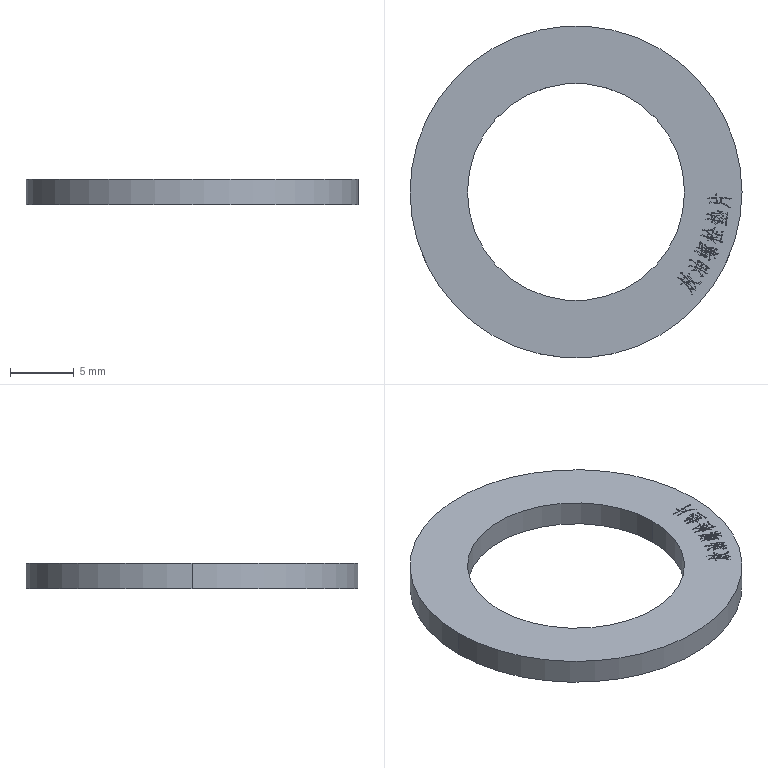Part | SolidWorks | features Extrusion 1, ICE 1 | 1 solid | 718 faces | box 26 x 26 x 2 mm | volume 607.665 mm3 | plane 543 | spline 171 | cylinder 4 | commonest cylinder face diameters 17 x2 26 x2